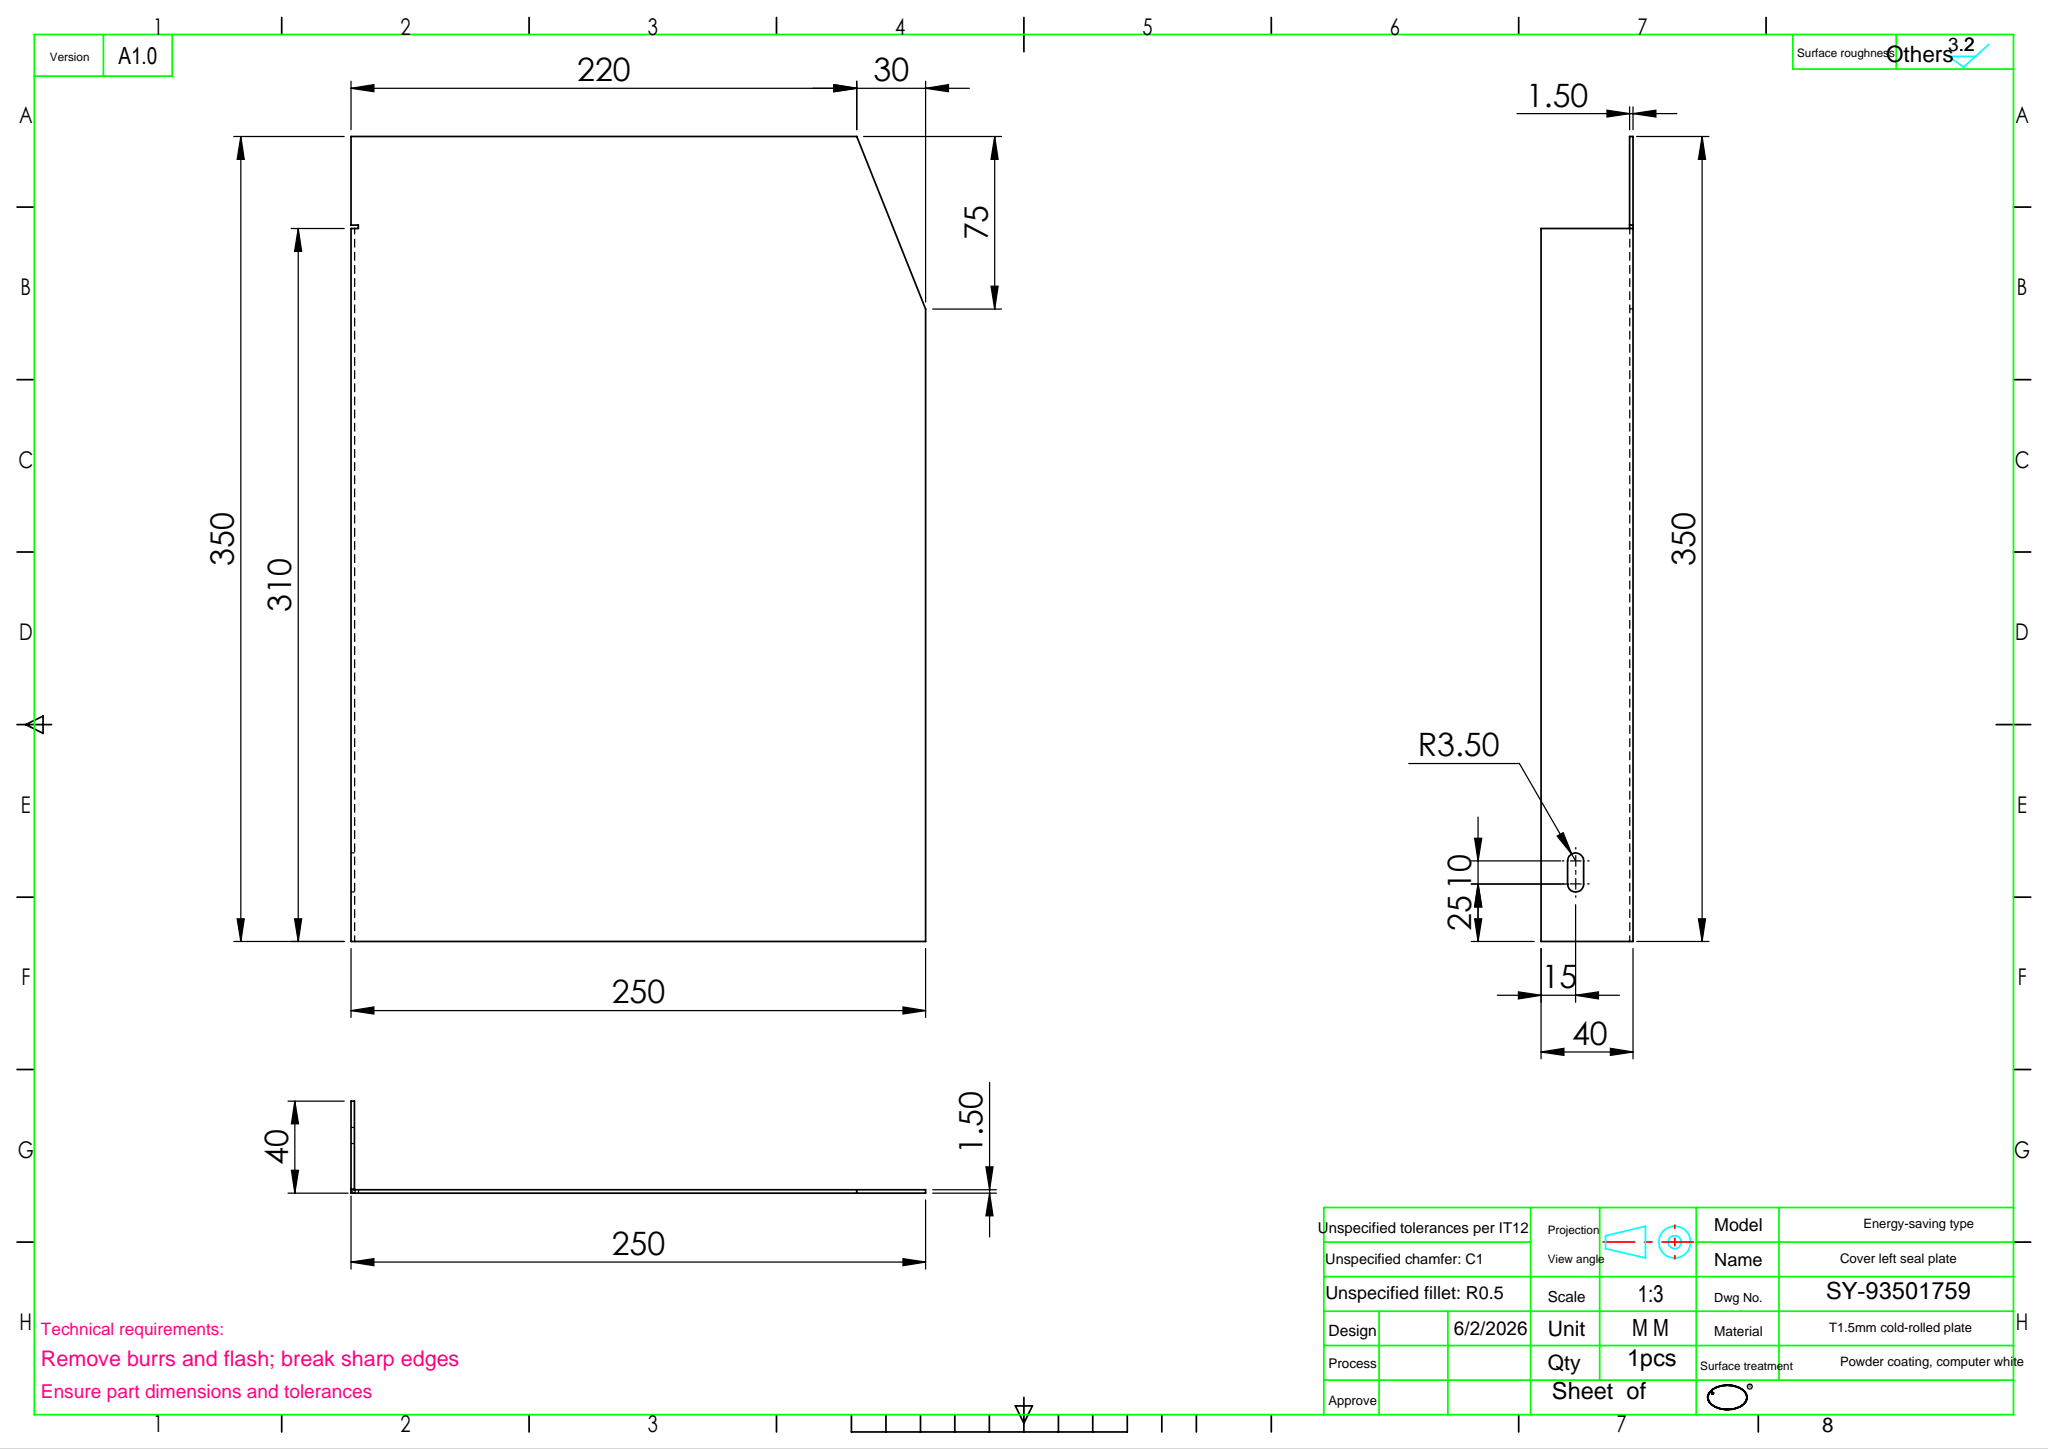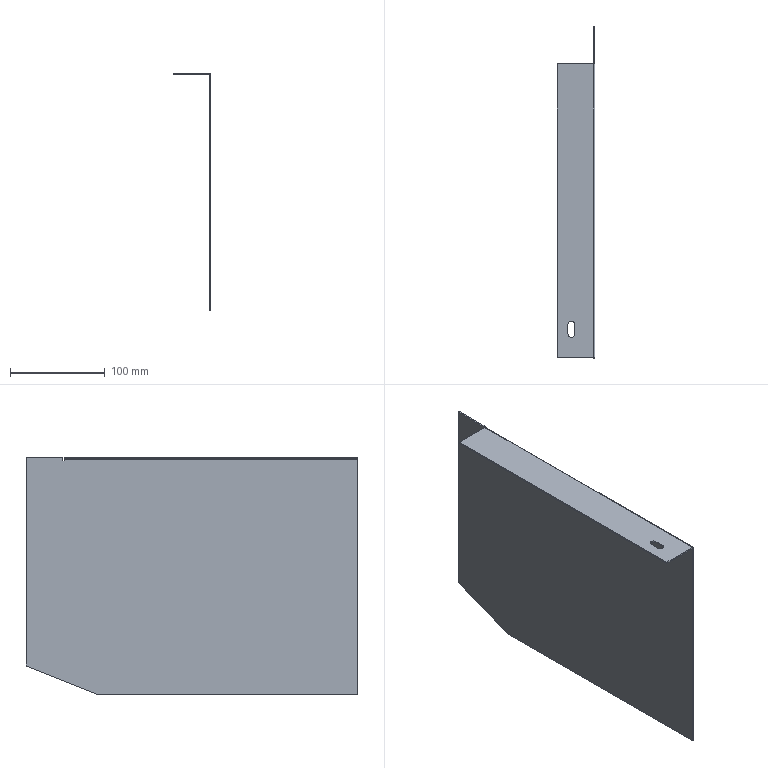Part | SolidWorks | features EdgeFlange 1, FlatPattern 1, ICE 1, SMBaseFlange 1, SheetMetal 1 | 1 solid | 24 faces | box 40 x 350 x 250 mm | volume 147105 mm3 | plane 19 | cylinder 5 | commonest cylinder face diameters 7 x3 0.4 x1 3.4 x1
STEP:
#1=CARTESIAN_POINT('',(-21.5,35.,0.));
#2=VERTEX_POINT('',#1);
#3=CARTESIAN_POINT('',(-25.,38.5,0.));
#4=VERTEX_POINT('',#3);
#5=CARTESIAN_POINT('',(-25.,35.,0.));
#6=DIRECTION('',(0.,0.,1.));
#7=DIRECTION('',(1.,0.,0.));
#8=AXIS2_PLACEMENT_3D('',#5,#6,#7);
#9=CIRCLE('',#8,3.5);
#10=EDGE_CURVE('',#2,#4,#9,.T.);
#11=ORIENTED_EDGE('',*,*,#10,.T.);
#12=CARTESIAN_POINT('',(-25.,38.5,-1.5));
#13=VERTEX_POINT('',#12);
#14=CARTESIAN_POINT('',(-25.,38.5,8.5));
#15=DIRECTION('',(0.,0.,-1.));
#16=VECTOR('',#15,1000.);
#17=LINE('',#14,#16);
#18=EDGE_CURVE('',#4,#13,#17,.T.);
#19=ORIENTED_EDGE('',*,*,#18,.T.);
#20=CARTESIAN_POINT('',(-21.5,35.,-1.5));
#21=VERTEX_POINT('',#20);
#22=CARTESIAN_POINT('',(-25.,35.,-1.5));
#23=DIRECTION('',(0.,0.,-1.));
#24=DIRECTION('',(0.,1.,0.));
#25=AXIS2_PLACEMENT_3D('',#22,#23,#24);
#26=CIRCLE('',#25,3.5);
#27=EDGE_CURVE('',#13,#21,#26,.T.);
#28=ORIENTED_EDGE('',*,*,#27,.T.);
#29=CARTESIAN_POINT('',(-21.5,35.,8.5));
#30=DIRECTION('',(0.,0.,-1.));
#31=VECTOR('',#30,1000.);
#32=LINE('',#29,#31);
#33=EDGE_CURVE('',#2,#21,#32,.T.);
#34=ORIENTED_EDGE('',*,*,#33,.F.);
#35=EDGE_LOOP('',(#11,#19,#28,#34));
#36=FACE_OUTER_BOUND('',#35,.T.);
#37=CARTESIAN_POINT('',(-25.,35.,8.5));
#38=DIRECTION('',(0.,0.,-1.));
#39=DIRECTION('',(0.,1.,0.));
#40=AXIS2_PLACEMENT_3D('',#37,#38,#39);
#41=CYLINDRICAL_SURFACE('',#40,3.5);
#42=ADVANCED_FACE('',(#36),#41,.F.);
#43=CARTESIAN_POINT('',(-1.5,350.,0.));
#44=VERTEX_POINT('',#43);
#45=CARTESIAN_POINT('',(-1.5,311.5,0.));
#46=VERTEX_POINT('',#45);
#47=CARTESIAN_POINT('',(-1.5,350.,0.));
#48=DIRECTION('',(0.,-1.,0.));
#49=VECTOR('',#48,1000.);
#50=LINE('',#47,#49);
#51=EDGE_CURVE('',#44,#46,#50,.T.);
#52=ORIENTED_EDGE('',*,*,#51,.T.);
#53=CARTESIAN_POINT('',(0.,311.5,0.));
#54=VERTEX_POINT('',#53);
#55=CARTESIAN_POINT('',(-1.5,311.5,0.));
#56=DIRECTION('',(1.,0.,0.));
#57=VECTOR('',#56,1000.);
#58=LINE('',#55,#57);
#59=EDGE_CURVE('',#46,#54,#58,.T.);
#60=ORIENTED_EDGE('',*,*,#59,.T.);
#61=CARTESIAN_POINT('',(0.,350.,0.));
#62=VERTEX_POINT('',#61);
#63=CARTESIAN_POINT('',(0.,350.,0.));
#64=DIRECTION('',(0.,-1.,0.));
#65=VECTOR('',#64,1000.);
#66=LINE('',#63,#65);
#67=EDGE_CURVE('',#62,#54,#66,.T.);
#68=ORIENTED_EDGE('',*,*,#67,.F.);
#69=CARTESIAN_POINT('',(-1.5,350.,0.));
#70=DIRECTION('',(1.,0.,0.));
#71=VECTOR('',#70,1000.);
#72=LINE('',#69,#71);
#73=EDGE_CURVE('',#44,#62,#72,.T.);
#74=ORIENTED_EDGE('',*,*,#73,.F.);
#75=EDGE_LOOP('',(#52,#60,#68,#74));
#76=FACE_OUTER_BOUND('',#75,.T.);
#77=CARTESIAN_POINT('',(-1.5,350.,0.));
#78=DIRECTION('',(0.,0.,1.));
#79=DIRECTION('',(0.,-1.,0.));
#80=AXIS2_PLACEMENT_3D('',#77,#78,#79);
#81=PLANE('',#80);
#82=ADVANCED_FACE('',(#76),#81,.T.);
#83=CARTESIAN_POINT('',(-1.5,311.5,-3.2));
#84=VERTEX_POINT('',#83);
#85=CARTESIAN_POINT('',(-1.5,311.5,0.));
#86=DIRECTION('',(0.,0.,-1.));
#87=VECTOR('',#86,1000.);
#88=LINE('',#85,#87);
#89=EDGE_CURVE('',#46,#84,#88,.T.);
#90=ORIENTED_EDGE('',*,*,#89,.F.);
#91=ORIENTED_EDGE('',*,*,#51,.F.);
#92=CARTESIAN_POINT('',(-1.5,350.,-220.));
#93=VERTEX_POINT('',#92);
#94=CARTESIAN_POINT('',(-1.5,350.,0.));
#95=DIRECTION('',(0.,0.,1.));
#96=VECTOR('',#95,1000.);
#97=LINE('',#94,#96);
#98=EDGE_CURVE('',#93,#44,#97,.T.);
#99=ORIENTED_EDGE('',*,*,#98,.F.);
#100=CARTESIAN_POINT('',(-1.5,275.,-250.));
#101=VERTEX_POINT('',#100);
#102=CARTESIAN_POINT('',(-1.5,350.,-220.));
#103=DIRECTION('',(0.,0.9285,0.3714));
#104=VECTOR('',#103,1000.);
#105=LINE('',#102,#104);
#106=EDGE_CURVE('',#101,#93,#105,.T.);
#107=ORIENTED_EDGE('',*,*,#106,.F.);
#108=CARTESIAN_POINT('',(-1.5,0.,-250.));
#109=VERTEX_POINT('',#108);
#110=CARTESIAN_POINT('',(-1.5,275.,-250.));
#111=DIRECTION('',(0.,1.,0.));
#112=VECTOR('',#111,1000.);
#113=LINE('',#110,#112);
#114=EDGE_CURVE('',#109,#101,#113,.T.);
#115=ORIENTED_EDGE('',*,*,#114,.F.);
#116=CARTESIAN_POINT('',(-1.5,0.,-1.7));
#117=VERTEX_POINT('',#116);
#118=CARTESIAN_POINT('',(-1.5,0.,0.));
#119=DIRECTION('',(0.,0.,-1.));
#120=VECTOR('',#119,1000.);
#121=LINE('',#118,#120);
#122=EDGE_CURVE('',#117,#109,#121,.T.);
#123=ORIENTED_EDGE('',*,*,#122,.F.);
#124=CARTESIAN_POINT('',(-1.5,310.,-1.7));
#125=VERTEX_POINT('',#124);
#126=CARTESIAN_POINT('',(-1.5,310.,-1.7));
#127=DIRECTION('',(0.,-1.,0.));
#128=VECTOR('',#127,1000.);
#129=LINE('',#126,#128);
#130=EDGE_CURVE('',#125,#117,#129,.T.);
#131=ORIENTED_EDGE('',*,*,#130,.F.);
#132=CARTESIAN_POINT('',(-1.5,310.,-3.2));
#133=VERTEX_POINT('',#132);
#134=CARTESIAN_POINT('',(-1.5,310.,-3.2));
#135=DIRECTION('',(0.,0.,1.));
#136=VECTOR('',#135,1000.);
#137=LINE('',#134,#136);
#138=EDGE_CURVE('',#133,#125,#137,.T.);
#139=ORIENTED_EDGE('',*,*,#138,.F.);
#140=CARTESIAN_POINT('',(-1.5,311.5,-3.2));
#141=DIRECTION('',(0.,-1.,0.));
#142=VECTOR('',#141,1000.);
#143=LINE('',#140,#142);
#144=EDGE_CURVE('',#84,#133,#143,.T.);
#145=ORIENTED_EDGE('',*,*,#144,.F.);
#146=EDGE_LOOP('',(#90,#91,#99,#107,#115,#123,#131,#139,#145));
#147=FACE_OUTER_BOUND('',#146,.T.);
#148=CARTESIAN_POINT('',(-1.5,0.,0.));
#149=DIRECTION('',(1.,0.,0.));
#150=DIRECTION('',(0.,0.,-1.));
#151=AXIS2_PLACEMENT_3D('',#148,#149,#150);
#152=PLANE('',#151);
#153=ADVANCED_FACE('',(#147),#152,.F.);
#154=ORIENTED_EDGE('',*,*,#67,.T.);
#155=CARTESIAN_POINT('',(0.,311.5,-3.2));
#156=VERTEX_POINT('',#155);
#157=CARTESIAN_POINT('',(0.,311.5,0.));
#158=DIRECTION('',(0.,0.,-1.));
#159=VECTOR('',#158,1000.);
#160=LINE('',#157,#159);
#161=EDGE_CURVE('',#54,#156,#160,.T.);
#162=ORIENTED_EDGE('',*,*,#161,.T.);
#163=CARTESIAN_POINT('',(0.,310.,-3.2));
#164=VERTEX_POINT('',#163);
#165=CARTESIAN_POINT('',(0.,0.,-3.2));
#166=DIRECTION('',(0.,-1.,0.));
#167=VECTOR('',#166,1000.);
#168=LINE('',#165,#167);
#169=EDGE_CURVE('',#156,#164,#168,.T.);
#170=ORIENTED_EDGE('',*,*,#169,.T.);
#171=CARTESIAN_POINT('',(0.,310.,-1.7));
#172=VERTEX_POINT('',#171);
#173=CARTESIAN_POINT('',(0.,310.,0.));
#174=DIRECTION('',(0.,0.,1.));
#175=VECTOR('',#174,1000.);
#176=LINE('',#173,#175);
#177=EDGE_CURVE('',#164,#172,#176,.T.);
#178=ORIENTED_EDGE('',*,*,#177,.T.);
#179=CARTESIAN_POINT('',(0.,0.,-1.7));
#180=VERTEX_POINT('',#179);
#181=CARTESIAN_POINT('',(0.,310.,-1.7));
#182=DIRECTION('',(0.,-1.,0.));
#183=VECTOR('',#182,1000.);
#184=LINE('',#181,#183);
#185=EDGE_CURVE('',#172,#180,#184,.T.);
#186=ORIENTED_EDGE('',*,*,#185,.T.);
#187=CARTESIAN_POINT('',(0.,0.,-250.));
#188=VERTEX_POINT('',#187);
#189=CARTESIAN_POINT('',(0.,0.,0.));
#190=DIRECTION('',(0.,0.,-1.));
#191=VECTOR('',#190,1000.);
#192=LINE('',#189,#191);
#193=EDGE_CURVE('',#180,#188,#192,.T.);
#194=ORIENTED_EDGE('',*,*,#193,.T.);
#195=CARTESIAN_POINT('',(0.,275.,-250.));
#196=VERTEX_POINT('',#195);
#197=CARTESIAN_POINT('',(0.,275.,-250.));
#198=DIRECTION('',(0.,1.,0.));
#199=VECTOR('',#198,1000.);
#200=LINE('',#197,#199);
#201=EDGE_CURVE('',#188,#196,#200,.T.);
#202=ORIENTED_EDGE('',*,*,#201,.T.);
#203=CARTESIAN_POINT('',(0.,350.,-220.));
#204=VERTEX_POINT('',#203);
#205=CARTESIAN_POINT('',(0.,350.,-220.));
#206=DIRECTION('',(0.,0.9285,0.3714));
#207=VECTOR('',#206,1000.);
#208=LINE('',#205,#207);
#209=EDGE_CURVE('',#196,#204,#208,.T.);
#210=ORIENTED_EDGE('',*,*,#209,.T.);
#211=CARTESIAN_POINT('',(0.,350.,0.));
#212=DIRECTION('',(0.,0.,1.));
#213=VECTOR('',#212,1000.);
#214=LINE('',#211,#213);
#215=EDGE_CURVE('',#204,#62,#214,.T.);
#216=ORIENTED_EDGE('',*,*,#215,.T.);
#217=EDGE_LOOP('',(#154,#162,#170,#178,#186,#194,#202,#210,#216));
#218=FACE_OUTER_BOUND('',#217,.T.);
#219=CARTESIAN_POINT('',(0.,0.,0.));
#220=DIRECTION('',(1.,0.,0.));
#221=DIRECTION('',(0.,0.,-1.));
#222=AXIS2_PLACEMENT_3D('',#219,#220,#221);
#223=PLANE('',#222);
#224=ADVANCED_FACE('',(#218),#223,.T.);
#225=ORIENTED_EDGE('',*,*,#215,.F.);
#226=CARTESIAN_POINT('',(-1.5,350.,-220.));
#227=DIRECTION('',(1.,0.,0.));
#228=VECTOR('',#227,1000.);
#229=LINE('',#226,#228);
#230=EDGE_CURVE('',#93,#204,#229,.T.);
#231=ORIENTED_EDGE('',*,*,#230,.F.);
#232=ORIENTED_EDGE('',*,*,#98,.T.);
#233=ORIENTED_EDGE('',*,*,#73,.T.);
#234=EDGE_LOOP('',(#225,#231,#232,#233));
#235=FACE_OUTER_BOUND('',#234,.T.);
#236=CARTESIAN_POINT('',(-1.5,350.,0.));
#237=DIRECTION('',(0.,1.,0.));
#238=DIRECTION('',(0.,0.,1.));
#239=AXIS2_PLACEMENT_3D('',#236,#237,#238);
#240=PLANE('',#239);
#241=ADVANCED_FACE('',(#235),#240,.T.);
#242=ORIENTED_EDGE('',*,*,#209,.F.);
#243=CARTESIAN_POINT('',(-1.5,275.,-250.));
#244=DIRECTION('',(1.,0.,0.));
#245=VECTOR('',#244,1000.);
#246=LINE('',#243,#245);
#247=EDGE_CURVE('',#101,#196,#246,.T.);
#248=ORIENTED_EDGE('',*,*,#247,.F.);
#249=ORIENTED_EDGE('',*,*,#106,.T.);
#250=ORIENTED_EDGE('',*,*,#230,.T.);
#251=EDGE_LOOP('',(#242,#248,#249,#250));
#252=FACE_OUTER_BOUND('',#251,.T.);
#253=CARTESIAN_POINT('',(-1.5,350.,-220.));
#254=DIRECTION('',(0.,0.3714,-0.9285));
#255=DIRECTION('',(0.,0.9285,0.3714));
#256=AXIS2_PLACEMENT_3D('',#253,#254,#255);
#257=PLANE('',#256);
#258=ADVANCED_FACE('',(#252),#257,.T.);
#259=ORIENTED_EDGE('',*,*,#201,.F.);
#260=CARTESIAN_POINT('',(-1.5,0.,-250.));
#261=DIRECTION('',(1.,0.,0.));
#262=VECTOR('',#261,1000.);
#263=LINE('',#260,#262);
#264=EDGE_CURVE('',#109,#188,#263,.T.);
#265=ORIENTED_EDGE('',*,*,#264,.F.);
#266=ORIENTED_EDGE('',*,*,#114,.T.);
#267=ORIENTED_EDGE('',*,*,#247,.T.);
#268=EDGE_LOOP('',(#259,#265,#266,#267));
#269=FACE_OUTER_BOUND('',#268,.T.);
#270=CARTESIAN_POINT('',(-1.5,275.,-250.));
#271=DIRECTION('',(0.,0.,-1.));
#272=DIRECTION('',(0.,1.,0.));
#273=AXIS2_PLACEMENT_3D('',#270,#271,#272);
#274=PLANE('',#273);
#275=ADVANCED_FACE('',(#269),#274,.T.);
#276=CARTESIAN_POINT('',(-1.5,0.,-1.7));
#277=DIRECTION('',(1.,0.,0.));
#278=VECTOR('',#277,1000.);
#279=LINE('',#276,#278);
#280=EDGE_CURVE('',#117,#180,#279,.T.);
#281=ORIENTED_EDGE('',*,*,#280,.F.);
#282=ORIENTED_EDGE('',*,*,#122,.T.);
#283=ORIENTED_EDGE('',*,*,#264,.T.);
#284=ORIENTED_EDGE('',*,*,#193,.F.);
#285=EDGE_LOOP('',(#281,#282,#283,#284));
#286=FACE_OUTER_BOUND('',#285,.T.);
#287=CARTESIAN_POINT('',(-1.5,0.,0.));
#288=DIRECTION('',(0.,-1.,0.));
#289=DIRECTION('',(0.,0.,-1.));
#290=AXIS2_PLACEMENT_3D('',#287,#288,#289);
#291=PLANE('',#290);
#292=ADVANCED_FACE('',(#286),#291,.T.);
#293=ORIENTED_EDGE('',*,*,#161,.F.);
#294=ORIENTED_EDGE('',*,*,#59,.F.);
#295=ORIENTED_EDGE('',*,*,#89,.T.);
#296=CARTESIAN_POINT('',(-1.5,311.5,-3.2));
#297=DIRECTION('',(1.,0.,0.));
#298=VECTOR('',#297,1000.);
#299=LINE('',#296,#298);
#300=EDGE_CURVE('',#84,#156,#299,.T.);
#301=ORIENTED_EDGE('',*,*,#300,.T.);
#302=EDGE_LOOP('',(#293,#294,#295,#301));
#303=FACE_OUTER_BOUND('',#302,.T.);
#304=CARTESIAN_POINT('',(-1.5,311.5,0.));
#305=DIRECTION('',(0.,-1.,0.));
#306=DIRECTION('',(0.,0.,-1.));
#307=AXIS2_PLACEMENT_3D('',#304,#305,#306);
#308=PLANE('',#307);
#309=ADVANCED_FACE('',(#303),#308,.T.);
#310=ORIENTED_EDGE('',*,*,#169,.F.);
#311=ORIENTED_EDGE('',*,*,#300,.F.);
#312=ORIENTED_EDGE('',*,*,#144,.T.);
#313=CARTESIAN_POINT('',(-1.5,310.,-3.2));
#314=DIRECTION('',(1.,0.,0.));
#315=VECTOR('',#314,1000.);
#316=LINE('',#313,#315);
#317=EDGE_CURVE('',#133,#164,#316,.T.);
#318=ORIENTED_EDGE('',*,*,#317,.T.);
#319=EDGE_LOOP('',(#310,#311,#312,#318));
#320=FACE_OUTER_BOUND('',#319,.T.);
#321=CARTESIAN_POINT('',(-1.5,311.5,-3.2));
#322=DIRECTION('',(0.,0.,1.));
#323=DIRECTION('',(1.,0.,0.));
#324=AXIS2_PLACEMENT_3D('',#321,#322,#323);
#325=PLANE('',#324);
#326=ADVANCED_FACE('',(#320),#325,.T.);
#327=ORIENTED_EDGE('',*,*,#177,.F.);
#328=ORIENTED_EDGE('',*,*,#317,.F.);
#329=ORIENTED_EDGE('',*,*,#138,.T.);
#330=CARTESIAN_POINT('',(-1.5,310.,-1.7));
#331=DIRECTION('',(1.,0.,0.));
#332=VECTOR('',#331,1000.);
#333=LINE('',#330,#332);
#334=EDGE_CURVE('',#125,#172,#333,.T.);
#335=ORIENTED_EDGE('',*,*,#334,.T.);
#336=EDGE_LOOP('',(#327,#328,#329,#335));
#337=FACE_OUTER_BOUND('',#336,.T.);
#338=CARTESIAN_POINT('',(-1.5,310.,-3.2));
#339=DIRECTION('',(0.,1.,0.));
#340=DIRECTION('',(0.,0.,1.));
#341=AXIS2_PLACEMENT_3D('',#338,#339,#340);
#342=PLANE('',#341);
#343=ADVANCED_FACE('',(#337),#342,.T.);
#344=CARTESIAN_POINT('',(-1.7,0.,-1.5));
#345=VERTEX_POINT('',#344);
#346=CARTESIAN_POINT('',(-1.7,0.,0.));
#347=VERTEX_POINT('',#346);
#348=CARTESIAN_POINT('',(-1.7,0.,0.));
#349=DIRECTION('',(0.,0.,1.));
#350=VECTOR('',#349,1000.);
#351=LINE('',#348,#350);
#352=EDGE_CURVE('',#345,#347,#351,.T.);
#353=ORIENTED_EDGE('',*,*,#352,.F.);
#354=CARTESIAN_POINT('',(-1.7,0.,-1.7));
#355=DIRECTION('',(0.,-1.,0.));
#356=DIRECTION('',(0.,0.,1.));
#357=AXIS2_PLACEMENT_3D('',#354,#355,#356);
#358=CIRCLE('',#357,0.2);
#359=EDGE_CURVE('',#117,#345,#358,.T.);
#360=ORIENTED_EDGE('',*,*,#359,.F.);
#361=ORIENTED_EDGE('',*,*,#280,.T.);
#362=CARTESIAN_POINT('',(-1.7,0.,-1.7));
#363=DIRECTION('',(0.,-1.,0.));
#364=DIRECTION('',(0.,0.,1.));
#365=AXIS2_PLACEMENT_3D('',#362,#363,#364);
#366=CIRCLE('',#365,1.7);
#367=EDGE_CURVE('',#180,#347,#366,.T.);
#368=ORIENTED_EDGE('',*,*,#367,.T.);
#369=EDGE_LOOP('',(#353,#360,#361,#368));
#370=FACE_OUTER_BOUND('',#369,.T.);
#371=CARTESIAN_POINT('',(-1.7,0.,-1.7));
#372=DIRECTION('',(0.,-1.,0.));
#373=DIRECTION('',(0.,0.,-1.));
#374=AXIS2_PLACEMENT_3D('',#371,#372,#373);
#375=PLANE('',#374);
#376=ADVANCED_FACE('',(#370),#375,.T.);
#377=CARTESIAN_POINT('',(-1.7,310.,-1.5));
#378=VERTEX_POINT('',#377);
#379=CARTESIAN_POINT('',(-1.7,310.,-1.7));
#380=DIRECTION('',(0.,1.,0.));
#381=DIRECTION('',(0.,0.,1.));
#382=AXIS2_PLACEMENT_3D('',#379,#380,#381);
#383=CIRCLE('',#382,0.2);
#384=EDGE_CURVE('',#378,#125,#383,.T.);
#385=ORIENTED_EDGE('',*,*,#384,.F.);
#386=CARTESIAN_POINT('',(-1.7,310.,0.));
#387=VERTEX_POINT('',#386);
#388=CARTESIAN_POINT('',(-1.7,310.,-1.5));
#389=DIRECTION('',(0.,0.,1.));
#390=VECTOR('',#389,1000.);
#391=LINE('',#388,#390);
#392=EDGE_CURVE('',#378,#387,#391,.T.);
#393=ORIENTED_EDGE('',*,*,#392,.T.);
#394=CARTESIAN_POINT('',(-1.7,310.,-1.7));
#395=DIRECTION('',(0.,1.,0.));
#396=DIRECTION('',(0.,0.,1.));
#397=AXIS2_PLACEMENT_3D('',#394,#395,#396);
#398=CIRCLE('',#397,1.7);
#399=EDGE_CURVE('',#387,#172,#398,.T.);
#400=ORIENTED_EDGE('',*,*,#399,.T.);
#401=ORIENTED_EDGE('',*,*,#334,.F.);
#402=EDGE_LOOP('',(#385,#393,#400,#401));
#403=FACE_OUTER_BOUND('',#402,.T.);
#404=CARTESIAN_POINT('',(-1.7,310.,-1.7));
#405=DIRECTION('',(0.,-1.,0.));
#406=DIRECTION('',(0.,0.,-1.));
#407=AXIS2_PLACEMENT_3D('',#404,#405,#406);
#408=PLANE('',#407);
#409=ADVANCED_FACE('',(#403),#408,.F.);
#410=ORIENTED_EDGE('',*,*,#185,.F.);
#411=ORIENTED_EDGE('',*,*,#399,.F.);
#412=CARTESIAN_POINT('',(-1.7,0.,0.));
#413=DIRECTION('',(0.,1.,0.));
#414=VECTOR('',#413,1000.);
#415=LINE('',#412,#414);
#416=EDGE_CURVE('',#347,#387,#415,.T.);
#417=ORIENTED_EDGE('',*,*,#416,.F.);
#418=ORIENTED_EDGE('',*,*,#367,.F.);
#419=EDGE_LOOP('',(#410,#411,#417,#418));
#420=FACE_OUTER_BOUND('',#419,.T.);
#421=CARTESIAN_POINT('',(-1.7,310.,-1.7));
#422=DIRECTION('',(0.,1.,0.));
#423=DIRECTION('',(0.,0.,1.));
#424=AXIS2_PLACEMENT_3D('',#421,#422,#423);
#425=CYLINDRICAL_SURFACE('',#424,1.7);
#426=ADVANCED_FACE('',(#420),#425,.T.);
#427=ORIENTED_EDGE('',*,*,#130,.T.);
#428=ORIENTED_EDGE('',*,*,#359,.T.);
#429=CARTESIAN_POINT('',(-1.7,0.,-1.5));
#430=DIRECTION('',(0.,1.,0.));
#431=VECTOR('',#430,1000.);
#432=LINE('',#429,#431);
#433=EDGE_CURVE('',#345,#378,#432,.T.);
#434=ORIENTED_EDGE('',*,*,#433,.T.);
#435=ORIENTED_EDGE('',*,*,#384,.T.);
#436=EDGE_LOOP('',(#427,#428,#434,#435));
#437=FACE_OUTER_BOUND('',#436,.T.);
#438=CARTESIAN_POINT('',(-1.7,310.,-1.7));
#439=DIRECTION('',(0.,1.,0.));
#440=DIRECTION('',(0.,0.,1.));
#441=AXIS2_PLACEMENT_3D('',#438,#439,#440);
#442=CYLINDRICAL_SURFACE('',#441,0.2);
#443=ADVANCED_FACE('',(#437),#442,.F.);
#444=CARTESIAN_POINT('',(-40.,310.,0.));
#445=VERTEX_POINT('',#444);
#446=CARTESIAN_POINT('',(-1.5,310.,0.));
#447=DIRECTION('',(1.,0.,0.));
#448=VECTOR('',#447,1000.);
#449=LINE('',#446,#448);
#450=EDGE_CURVE('',#445,#387,#449,.T.);
#451=ORIENTED_EDGE('',*,*,#450,.T.);
#452=ORIENTED_EDGE('',*,*,#392,.F.);
#453=CARTESIAN_POINT('',(-40.,310.,-1.5));
#454=VERTEX_POINT('',#453);
#455=CARTESIAN_POINT('',(0.,310.,-1.5));
#456=DIRECTION('',(1.,0.,0.));
#457=VECTOR('',#456,1000.);
#458=LINE('',#455,#457);
#459=EDGE_CURVE('',#454,#378,#458,.T.);
#460=ORIENTED_EDGE('',*,*,#459,.F.);
#461=CARTESIAN_POINT('',(-40.,310.,0.));
#462=DIRECTION('',(0.,0.,-1.));
#463=VECTOR('',#462,1000.);
#464=LINE('',#461,#463);
#465=EDGE_CURVE('',#445,#454,#464,.T.);
#466=ORIENTED_EDGE('',*,*,#465,.F.);
#467=EDGE_LOOP('',(#451,#452,#460,#466));
#468=FACE_OUTER_BOUND('',#467,.T.);
#469=CARTESIAN_POINT('',(-1.5,310.,0.));
#470=DIRECTION('',(0.,1.,0.));
#471=DIRECTION('',(0.,0.,1.));
#472=AXIS2_PLACEMENT_3D('',#469,#470,#471);
#473=PLANE('',#472);
#474=ADVANCED_FACE('',(#468),#473,.T.);
#475=CARTESIAN_POINT('',(-40.,0.,-1.5));
#476=VERTEX_POINT('',#475);
#477=CARTESIAN_POINT('',(0.,0.,-1.5));
#478=DIRECTION('',(-1.,0.,0.));
#479=VECTOR('',#478,1000.);
#480=LINE('',#477,#479);
#481=EDGE_CURVE('',#345,#476,#480,.T.);
#482=ORIENTED_EDGE('',*,*,#481,.F.);
#483=ORIENTED_EDGE('',*,*,#352,.T.);
#484=CARTESIAN_POINT('',(-40.,0.,0.));
#485=VERTEX_POINT('',#484);
#486=CARTESIAN_POINT('',(-40.,0.,0.));
#487=DIRECTION('',(-1.,0.,0.));
#488=VECTOR('',#487,1000.);
#489=LINE('',#486,#488);
#490=EDGE_CURVE('',#347,#485,#489,.T.);
#491=ORIENTED_EDGE('',*,*,#490,.T.);
#492=CARTESIAN_POINT('',(-40.,0.,0.));
#493=DIRECTION('',(0.,0.,-1.));
#494=VECTOR('',#493,1000.);
#495=LINE('',#492,#494);
#496=EDGE_CURVE('',#485,#476,#495,.T.);
#497=ORIENTED_EDGE('',*,*,#496,.T.);
#498=EDGE_LOOP('',(#482,#483,#491,#497));
#499=FACE_OUTER_BOUND('',#498,.T.);
#500=CARTESIAN_POINT('',(-40.,0.,0.));
#501=DIRECTION('',(0.,-1.,0.));
#502=DIRECTION('',(0.,0.,-1.));
#503=AXIS2_PLACEMENT_3D('',#500,#501,#502);
#504=PLANE('',#503);
#505=ADVANCED_FACE('',(#499),#504,.T.);
#506=ORIENTED_EDGE('',*,*,#10,.F.);
#507=CARTESIAN_POINT('',(-21.5,25.,0.));
#508=VERTEX_POINT('',#507);
#509=CARTESIAN_POINT('',(-21.5,0.,0.));
#510=DIRECTION('',(0.,1.,0.));
#511=VECTOR('',#510,1000.);
#512=LINE('',#509,#511);
#513=EDGE_CURVE('',#508,#2,#512,.T.);
#514=ORIENTED_EDGE('',*,*,#513,.F.);
#515=CARTESIAN_POINT('',(-28.5,25.,0.));
#516=VERTEX_POINT('',#515);
#517=CARTESIAN_POINT('',(-25.,25.,0.));
#518=DIRECTION('',(0.,0.,1.));
#519=DIRECTION('',(1.,0.,0.));
#520=AXIS2_PLACEMENT_3D('',#517,#518,#519);
#521=CIRCLE('',#520,3.5);
#522=EDGE_CURVE('',#516,#508,#521,.T.);
#523=ORIENTED_EDGE('',*,*,#522,.F.);
#524=CARTESIAN_POINT('',(-28.5,35.,0.));
#525=VERTEX_POINT('',#524);
#526=CARTESIAN_POINT('',(-28.5,0.,0.));
#527=DIRECTION('',(0.,-1.,0.));
#528=VECTOR('',#527,1000.);
#529=LINE('',#526,#528);
#530=EDGE_CURVE('',#525,#516,#529,.T.);
#531=ORIENTED_EDGE('',*,*,#530,.F.);
#532=CARTESIAN_POINT('',(-25.,35.,0.));
#533=DIRECTION('',(0.,0.,1.));
#534=DIRECTION('',(1.,0.,0.));
#535=AXIS2_PLACEMENT_3D('',#532,#533,#534);
#536=CIRCLE('',#535,3.5);
#537=EDGE_CURVE('',#4,#525,#536,.T.);
#538=ORIENTED_EDGE('',*,*,#537,.F.);
#539=EDGE_LOOP('',(#506,#514,#523,#531,#538));
#540=FACE_BOUND('',#539,.T.);
#541=ORIENTED_EDGE('',*,*,#490,.F.);
#542=ORIENTED_EDGE('',*,*,#416,.T.);
#543=ORIENTED_EDGE('',*,*,#450,.F.);
#544=CARTESIAN_POINT('',(-40.,310.,0.));
#545=DIRECTION('',(0.,1.,0.));
#546=VECTOR('',#545,1000.);
#547=LINE('',#544,#546);
#548=EDGE_CURVE('',#485,#445,#547,.T.);
#549=ORIENTED_EDGE('',*,*,#548,.F.);
#550=EDGE_LOOP('',(#541,#542,#543,#549));
#551=FACE_OUTER_BOUND('',#550,.T.);
#552=CARTESIAN_POINT('',(0.,0.,0.));
#553=DIRECTION('',(0.,0.,1.));
#554=DIRECTION('',(1.,0.,0.));
#555=AXIS2_PLACEMENT_3D('',#552,#553,#554);
#556=PLANE('',#555);
#557=ADVANCED_FACE('',(#540,#551),#556,.T.);
#558=CARTESIAN_POINT('',(-21.5,25.,-1.5));
#559=VERTEX_POINT('',#558);
#560=CARTESIAN_POINT('',(-21.5,35.,-1.5));
#561=DIRECTION('',(0.,-1.,0.));
#562=VECTOR('',#561,1000.);
#563=LINE('',#560,#562);
#564=EDGE_CURVE('',#21,#559,#563,.T.);
#565=ORIENTED_EDGE('',*,*,#564,.F.);
#566=ORIENTED_EDGE('',*,*,#27,.F.);
#567=CARTESIAN_POINT('',(-28.5,35.,-1.5));
#568=VERTEX_POINT('',#567);
#569=CARTESIAN_POINT('',(-25.,35.,-1.5));
#570=DIRECTION('',(0.,0.,-1.));
#571=DIRECTION('',(0.,1.,0.));
#572=AXIS2_PLACEMENT_3D('',#569,#570,#571);
#573=CIRCLE('',#572,3.5);
#574=EDGE_CURVE('',#568,#13,#573,.T.);
#575=ORIENTED_EDGE('',*,*,#574,.F.);
#576=CARTESIAN_POINT('',(-28.5,25.,-1.5));
#577=VERTEX_POINT('',#576);
#578=CARTESIAN_POINT('',(-28.5,35.,-1.5));
#579=DIRECTION('',(0.,1.,0.));
#580=VECTOR('',#579,1000.);
#581=LINE('',#578,#580);
#582=EDGE_CURVE('',#577,#568,#581,.T.);
#583=ORIENTED_EDGE('',*,*,#582,.F.);
#584=CARTESIAN_POINT('',(-25.,25.,-1.5));
#585=DIRECTION('',(0.,0.,-1.));
#586=DIRECTION('',(0.,1.,0.));
#587=AXIS2_PLACEMENT_3D('',#584,#585,#586);
#588=CIRCLE('',#587,3.5);
#589=EDGE_CURVE('',#559,#577,#588,.T.);
#590=ORIENTED_EDGE('',*,*,#589,.F.);
#591=EDGE_LOOP('',(#565,#566,#575,#583,#590));
#592=FACE_BOUND('',#591,.T.);
#593=ORIENTED_EDGE('',*,*,#433,.F.);
#594=ORIENTED_EDGE('',*,*,#481,.T.);
#595=CARTESIAN_POINT('',(-40.,0.,-1.5));
#596=DIRECTION('',(0.,1.,0.));
#597=VECTOR('',#596,1000.);
#598=LINE('',#595,#597);
#599=EDGE_CURVE('',#476,#454,#598,.T.);
#600=ORIENTED_EDGE('',*,*,#599,.T.);
#601=ORIENTED_EDGE('',*,*,#459,.T.);
#602=EDGE_LOOP('',(#593,#594,#600,#601));
#603=FACE_OUTER_BOUND('',#602,.T.);
#604=CARTESIAN_POINT('',(0.,0.,-1.5));
#605=DIRECTION('',(0.,0.,1.));
#606=DIRECTION('',(1.,0.,0.));
#607=AXIS2_PLACEMENT_3D('',#604,#605,#606);
#608=PLANE('',#607);
#609=ADVANCED_FACE('',(#592,#603),#608,.F.);
#610=ORIENTED_EDGE('',*,*,#599,.F.);
#611=ORIENTED_EDGE('',*,*,#496,.F.);
#612=ORIENTED_EDGE('',*,*,#548,.T.);
#613=ORIENTED_EDGE('',*,*,#465,.T.);
#614=EDGE_LOOP('',(#610,#611,#612,#613));
#615=FACE_OUTER_BOUND('',#614,.T.);
#616=CARTESIAN_POINT('',(-40.,310.,0.));
#617=DIRECTION('',(-1.,0.,0.));
#618=DIRECTION('',(0.,0.,1.));
#619=AXIS2_PLACEMENT_3D('',#616,#617,#618);
#620=PLANE('',#619);
#621=ADVANCED_FACE('',(#615),#620,.T.);
#622=ORIENTED_EDGE('',*,*,#18,.F.);
#623=ORIENTED_EDGE('',*,*,#537,.T.);
#624=CARTESIAN_POINT('',(-28.5,35.,8.5));
#625=DIRECTION('',(0.,0.,-1.));
#626=VECTOR('',#625,1000.);
#627=LINE('',#624,#626);
#628=EDGE_CURVE('',#525,#568,#627,.T.);
#629=ORIENTED_EDGE('',*,*,#628,.T.);
#630=ORIENTED_EDGE('',*,*,#574,.T.);
#631=EDGE_LOOP('',(#622,#623,#629,#630));
#632=FACE_OUTER_BOUND('',#631,.T.);
#633=CARTESIAN_POINT('',(-25.,35.,8.5));
#634=DIRECTION('',(0.,0.,-1.));
#635=DIRECTION('',(0.,1.,0.));
#636=AXIS2_PLACEMENT_3D('',#633,#634,#635);
#637=CYLINDRICAL_SURFACE('',#636,3.5);
#638=ADVANCED_FACE('',(#632),#637,.F.);
#639=ORIENTED_EDGE('',*,*,#530,.T.);
#640=CARTESIAN_POINT('',(-28.5,25.,8.5));
#641=DIRECTION('',(0.,0.,-1.));
#642=VECTOR('',#641,1000.);
#643=LINE('',#640,#642);
#644=EDGE_CURVE('',#516,#577,#643,.T.);
#645=ORIENTED_EDGE('',*,*,#644,.T.);
#646=ORIENTED_EDGE('',*,*,#582,.T.);
#647=ORIENTED_EDGE('',*,*,#628,.F.);
#648=EDGE_LOOP('',(#639,#645,#646,#647));
#649=FACE_OUTER_BOUND('',#648,.T.);
#650=CARTESIAN_POINT('',(-28.5,35.,8.5));
#651=DIRECTION('',(-1.,0.,0.));
#652=DIRECTION('',(0.,-1.,0.));
#653=AXIS2_PLACEMENT_3D('',#650,#651,#652);
#654=PLANE('',#653);
#655=ADVANCED_FACE('',(#649),#654,.F.);
#656=ORIENTED_EDGE('',*,*,#522,.T.);
#657=CARTESIAN_POINT('',(-21.5,25.,8.5));
#658=DIRECTION('',(0.,0.,-1.));
#659=VECTOR('',#658,1000.);
#660=LINE('',#657,#659);
#661=EDGE_CURVE('',#508,#559,#660,.T.);
#662=ORIENTED_EDGE('',*,*,#661,.T.);
#663=ORIENTED_EDGE('',*,*,#589,.T.);
#664=ORIENTED_EDGE('',*,*,#644,.F.);
#665=EDGE_LOOP('',(#656,#662,#663,#664));
#666=FACE_OUTER_BOUND('',#665,.T.);
#667=CARTESIAN_POINT('',(-25.,25.,8.5));
#668=DIRECTION('',(0.,0.,-1.));
#669=DIRECTION('',(0.,1.,0.));
#670=AXIS2_PLACEMENT_3D('',#667,#668,#669);
#671=CYLINDRICAL_SURFACE('',#670,3.5);
#672=ADVANCED_FACE('',(#666),#671,.F.);
#673=ORIENTED_EDGE('',*,*,#513,.T.);
#674=ORIENTED_EDGE('',*,*,#33,.T.);
#675=ORIENTED_EDGE('',*,*,#564,.T.);
#676=ORIENTED_EDGE('',*,*,#661,.F.);
#677=EDGE_LOOP('',(#673,#674,#675,#676));
#678=FACE_OUTER_BOUND('',#677,.T.);
#679=CARTESIAN_POINT('',(-21.5,35.,8.5));
#680=DIRECTION('',(1.,0.,0.));
#681=DIRECTION('',(0.,1.,0.));
#682=AXIS2_PLACEMENT_3D('',#679,#680,#681);
#683=PLANE('',#682);
#684=ADVANCED_FACE('',(#678),#683,.F.);
#685=CLOSED_SHELL('',(#42,#82,#153,#224,#241,#258,#275,#292,#309,#326,#343,#376,#409,#426,#443,#474,#505,#557,#609,#621,#638,#655,#672,#684));
#686=MANIFOLD_SOLID_BREP('',#685);
#687=CARTESIAN_POINT('',(0.,0.,0.));
#688=DIRECTION('',(0.,0.,1.));
#689=DIRECTION('',(1.,0.,0.));
#690=AXIS2_PLACEMENT_3D('',#687,#688,#689);
#691=(LENGTH_UNIT()NAMED_UNIT(*)SI_UNIT(.MILLI.,.METRE.));
#692=UNCERTAINTY_MEASURE_WITH_UNIT(LENGTH_MEASURE(0.00001),#691,'','');
#693=(NAMED_UNIT(*)PLANE_ANGLE_UNIT()SI_UNIT($,.RADIAN.));
#694=(NAMED_UNIT(*)SI_UNIT($,.STERADIAN.)SOLID_ANGLE_UNIT());
#695=(GEOMETRIC_REPRESENTATION_CONTEXT(3)GLOBAL_UNCERTAINTY_ASSIGNED_CONTEXT((#692))GLOBAL_UNIT_ASSIGNED_CONTEXT((#691,#693,#694))REPRESENTATION_CONTEXT('',''));
#696=ADVANCED_BREP_SHAPE_REPRESENTATION('',(#686,#690),#695);